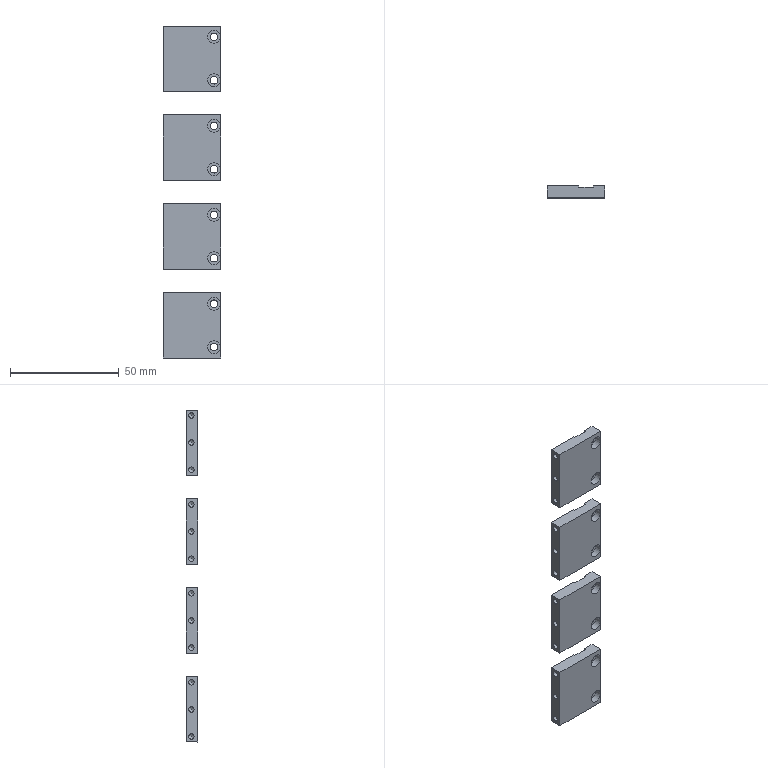CAM job | NX | 3+2 milling, drilling | part box 26.5 x 5.5 x 153 mm | stock box 31.5 x 8 x 158 mm
Tools:
number,name,description,diameter,corner_radius,flute_length,length,flutes
4,D4,平底铣刀-粗,4.0,0.0,25.0,75.0,2
9,D10,平底铣刀-粗,10.0,0.0,35.0,75.0,2
7,D6-J,平底铣刀-精,6.0,0.0,25.0,75.0,2
10,D10-J,平底铣刀-精,10.0,0.0,35.0,75.0,2
1,D80R0.8飞刀,圆鼻刀-粗,80.0,0.8,50.0,75.0,2
1,D80R0.8飞刀-J,圆鼻刀-精,80.0,0.8,50.0,75.0,2
2,D6倒角刀,倒角刀,6.0,0.0,3.0,25.0,2
17,ZT3.5,钻头,3.5,0.0,35.0,50.0,2
Operations:
program,operation,operation_type,tool,method,geometry_group,spindle_rpm,surface_speed,feed_per_tooth,feed_cut,feed_plunge,cut_length_mm,path_length_mm,cut_time_min,machine_time_min
B,底壁铣飞面一刀开粗_COPY,VolumeBased25DMillingOperation,D80R0.8飞刀,分层开粗-切深K-步距G,W-B,2800.0,703.696,0.5357,3000.0,100.0,1305.97,2403.948,0.4353,0.5451
B,底壁铣飞面一刀精光_COPY,VolumeBased25DMillingOperation,D80R0.8飞刀-J,侧刃精光-切深K-步距G,W-B,4000.0,1005.28,0.125,1000.0,100.0,260.998,296.998,0.261,0.2646
B,铣沉头_1,CylinderMilling,D4,METHOD,W-B,8000.0,100.531,0.075,1200.0,100.0,841.896,1346.496,0.7016,0.752
B,铣孔_1,CylinderMilling,D4,METHOD,W-B,8000.0,100.531,0.0375,600.0,100.0,74.078,605.078,0.1235,0.1766
B,平面去毛刺6X45L_COPY,SurfaceContour,D6倒角刀,爬面_倒角-切深0-步距G,W-B,6500.0,122.519,0.1154,1500.0,100.0,622.859,1172.759,0.4152,0.4702
A,顶面,FaceMilling,D80R0.8飞刀,侧刃精光-切深K-步距G,W-A,4000.0,1005.31,0.125,1000.0,100.0,247.0,283.0,0.247,0.2506
A,外形粗_2,VolumeBased25DMillingOperation,D10,METHOD,W-A,8000.0,251.327,0.3125,5000.0,80.0,5227.657,5525.557,1.046,1.075
A,打点-深0.8,Operation,D6倒角刀,NONE,W-A,8000.0,150.796,0.0312,500.0,90.0,14.4,218.971,0.0288,0.0493
A,通孔-3-4,Operation,ZT3.5,NONE,W-A,3000.0,32.987,0.02,120.0,90.0,72.0,334.171,0.6,0.6262
A,底壁粗_1,VolumeBased25DMillingOperation,D4,METHOD,W-A,6000.0,75.398,0.1,1200.0,100.0,876.0,1227.684,0.73,0.7652
A,仅选体,SurfaceContour,D6倒角刀,METHOD,W-A,8000.0,150.796,0.1875,3000.0,100.0,829.491,1864.239,0.2765,0.38
A,钻倒角_1,Operation,D6倒角刀,METHOD,W-A,8000.0,150.796,0.0312,500.0,0.0,40.4,286.335,0.0808,0.1054
A,底侧精_3,VolumeBased25DMillingOperation,D6-J,METHOD,W-A,6000.0,113.0,0.2083,1200.0,100.0,321.613,606.72,0.268,0.2965
A,外形半精_2,VolumeBased25DMillingOperation,D10-J,METHOD,W-A,8000.0,251.327,0.0625,1000.0,100.0,597.747,929.047,0.5977,0.6309